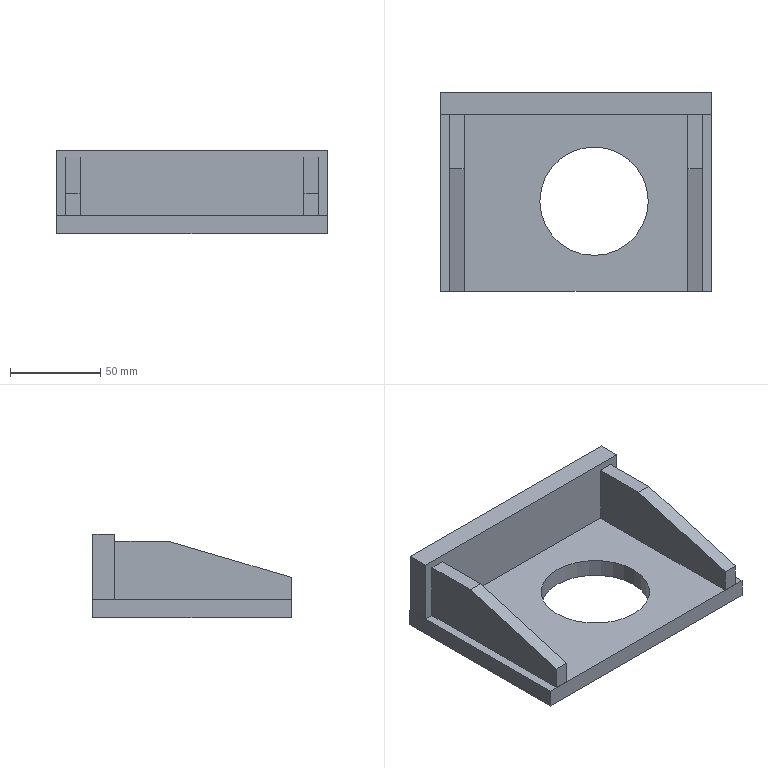Part | STEP file | PN_0013 | 1 solid | 25 faces | box 150 x 110 x 46.5 mm | volume 242294 mm3 | plane 23 | cylinder 2 | commonest cylinder face diameters 60 x2